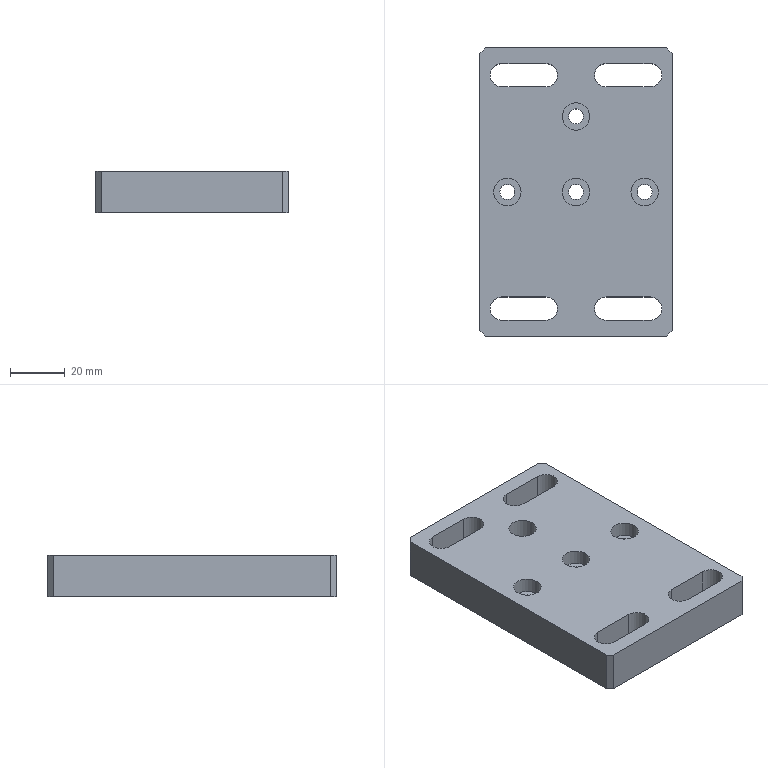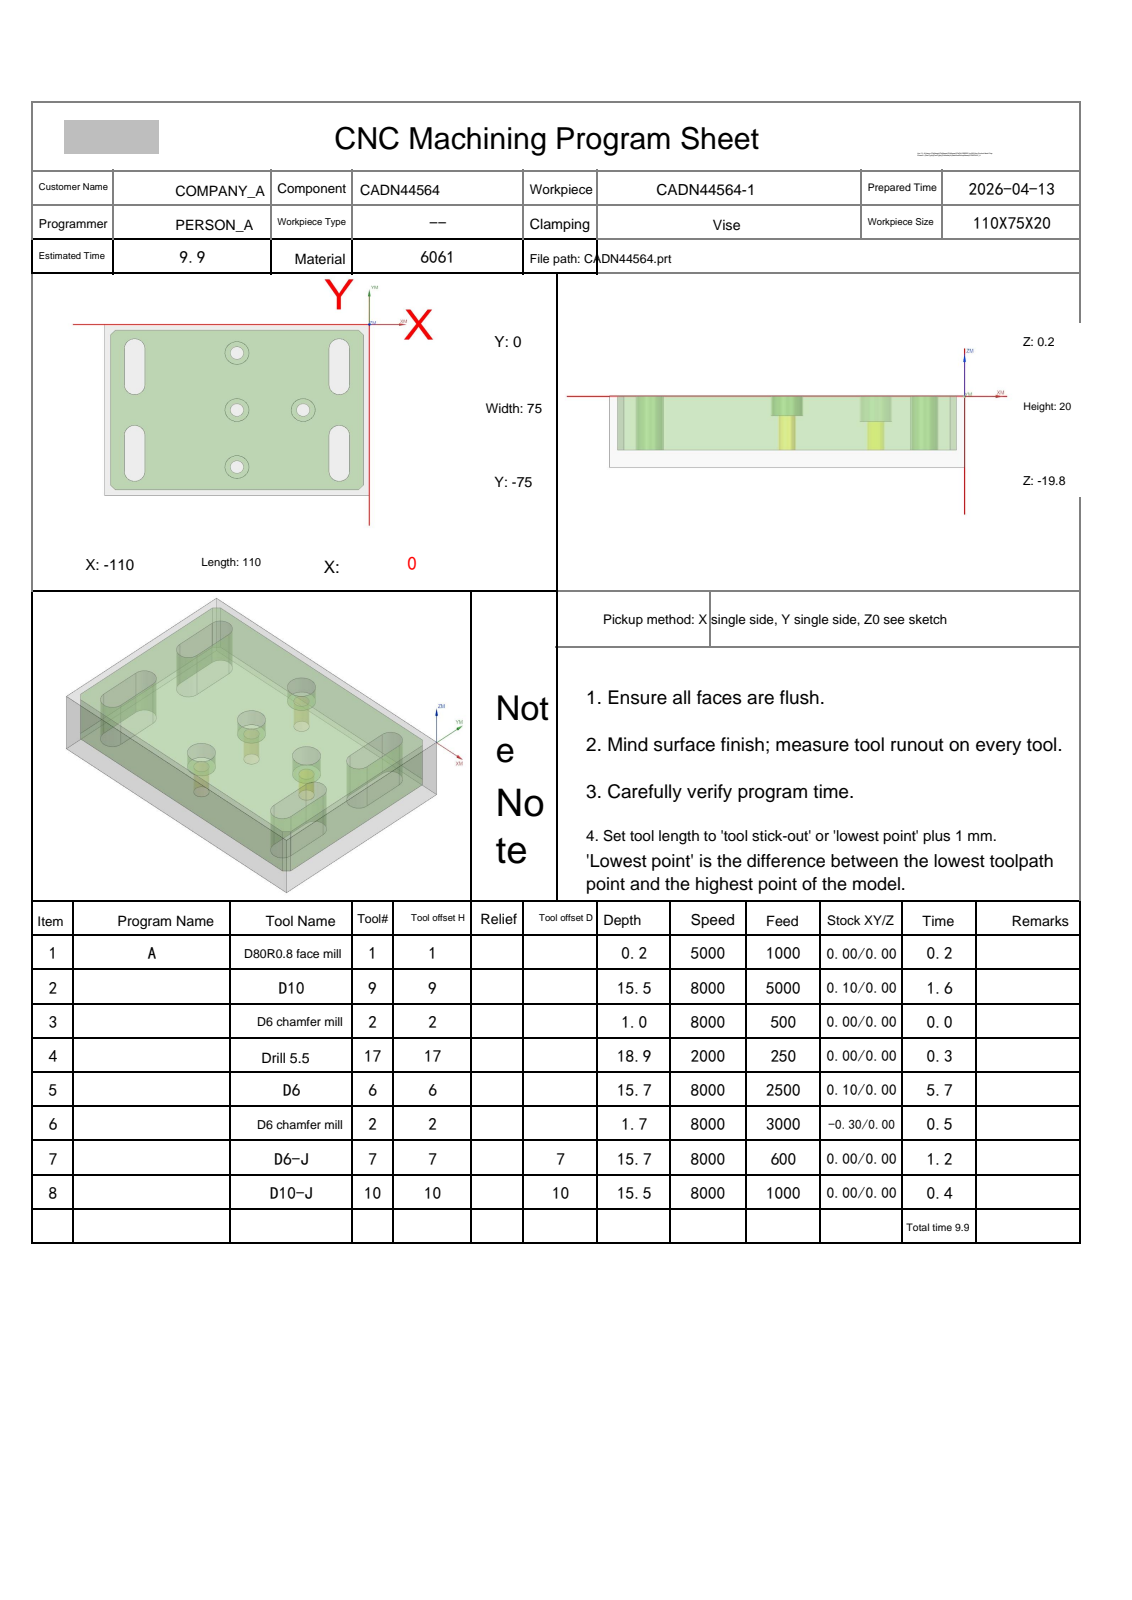NC program | NX | posted by the shop | part box 70 x 105 x 15 mm
Lines 1 to 417 of 3183:
%
O0001
(Machine time: 11.47 MIN)
(===Total Tool:7===)
(T1=D80R0.8 face mill D=80.  R=0.8  D-  H01 Z=0.    )
(T9=D10     D=10.  R=0.   D-  H09 Z=-15.3 )
(T2=D6 chamfer mill   D=6.   R=0.   D-  H02 Z=-1.5  )
(T17=Drill 5.5  D=5.5  DR_a=118 D-  H17 Z=-18.65)
(T6=D6      D=6.   R=0.   D-  H06 Z=-15.5 )
(T7=D6-J    D=6.   R=0.   D7  H07 Z=-15.5 )
(T10=D10-J  D=10.  R=0.   D10 H10 Z=-15.3 )
G80 G90 G17 G49 G40
G91 G28 Z0
M01
N1 T01 M06
(D80R0.8 face mill  D=80. R=0.8 H=01 ce=0.00 di=0.00)
G00 G90 G54 X-152.5 Y-37.5 M03 S5000
G43 H01 Z20.
M08
Z2.
G01 Z0.0 F1000.
X-147.5
X37.5
X42.5
Z2.
G00 Z20.
G91 G28 Z0.0
M05
M09
G91 G28 Z0.0
M01
N2 T09 M06
(D10  D=10. R=0. H=09 ce=0.10 di=0.00)
G00 G90 G54 X-55. Y-77.6 M03 S8000
G43 H09 Z20.
M08
Z.5
G01 X-105.5 Z.394 F5000.
G02 X-109.106 Y-76.106 Z.386 I0.0 J5.1
G01 X-111.106 Y-74.106 Z.38
G02 X-112.6 Y-70.5 Z.372 I3.606 J3.606
G01 Y-4.5 Z.233
G02 X-111.106 Y-.894 Z.225 I5.1 J0.0
G01 X-109.106 Y1.106 Z.219
G02 X-105.5 Y2.6 Z.211 I3.606 J-3.606
G01 X-4.5 Z-.001
G02 X-.894 Y1.106 Z-.009 I0.0 J-5.1
G01 X1.106 Y-.894 Z-.015
G02 X2.6 Y-4.5 Z-.023 I-3.606 J-3.606
G01 Y-70.5 Z-.162
G02 X1.106 Y-74.106 Z-.17 I-5.1 J0.0
G01 X-.894 Y-76.106 Z-.176
G02 X-4.5 Y-77.6 Z-.184 I-3.606 J3.606
G01 X-105.5 Z-.396
G02 X-109.106 Y-76.106 Z-.404 I0.0 J5.1
G01 X-111.106 Y-74.106 Z-.41
G02 X-112.6 Y-70.5 Z-.418 I3.606 J3.606
G01 Y-4.5 Z-.557
G02 X-111.106 Y-.894 Z-.565 I5.1 J0.0
G01 X-109.106 Y1.106 Z-.571
G02 X-105.5 Y2.6 Z-.579 I3.606 J-3.606
G01 X-4.5 Z-.791
G02 X-.894 Y1.106 Z-.799 I0.0 J-5.1
G01 X1.106 Y-.894 Z-.805
G02 X2.6 Y-4.5 Z-.813 I-3.606 J-3.606
G01 Y-70.5 Z-.952
G02 X1.106 Y-74.106 Z-.96 I-5.1 J0.0
G01 X-.894 Y-76.106 Z-.966
G02 X-4.5 Y-77.6 Z-.974 I-3.606 J3.606
G01 X-105.5 Z-1.186
G02 X-109.106 Y-76.106 Z-1.194 I0.0 J5.1
G01 X-111.106 Y-74.106 Z-1.2
G02 X-112.6 Y-70.5 Z-1.208 I3.606 J3.606
G01 Y-4.5 Z-1.347
G02 X-111.106 Y-.894 Z-1.355 I5.1 J0.0
G01 X-109.106 Y1.106 Z-1.361
G02 X-105.5 Y2.6 Z-1.369 I3.606 J-3.606
G01 X-4.5 Z-1.581
G02 X-.894 Y1.106 Z-1.589 I0.0 J-5.1
G01 X1.106 Y-.894 Z-1.595
G02 X2.6 Y-4.5 Z-1.603 I-3.606 J-3.606
G01 Y-70.5 Z-1.742
G02 X1.106 Y-74.106 Z-1.75 I-5.1 J0.0
G01 X-.894 Y-76.106 Z-1.756
G02 X-4.5 Y-77.6 Z-1.764 I-3.606 J3.606
G01 X-105.5 Z-1.976
G02 X-109.106 Y-76.106 Z-1.984 I0.0 J5.1
G01 X-111.106 Y-74.106 Z-1.99
G02 X-112.6 Y-70.5 Z-1.998 I3.606 J3.606
G01 Y-4.5 Z-2.137
G02 X-111.106 Y-.894 Z-2.145 I5.1 J0.0
G01 X-109.106 Y1.106 Z-2.151
G02 X-105.5 Y2.6 Z-2.159 I3.606 J-3.606
G01 X-4.5 Z-2.371
G02 X-.894 Y1.106 Z-2.379 I0.0 J-5.1
G01 X1.106 Y-.894 Z-2.385
G02 X2.6 Y-4.5 Z-2.393 I-3.606 J-3.606
G01 Y-70.5 Z-2.532
G02 X1.106 Y-74.106 Z-2.54 I-5.1 J0.0
G01 X-.894 Y-76.106 Z-2.546
G02 X-4.5 Y-77.6 Z-2.554 I-3.606 J3.606
G01 X-105.5 Z-2.766
G02 X-109.106 Y-76.106 Z-2.774 I0.0 J5.1
G01 X-111.106 Y-74.106 Z-2.78
G02 X-112.6 Y-70.5 Z-2.788 I3.606 J3.606
G01 Y-4.5 Z-2.927
G02 X-111.106 Y-.894 Z-2.935 I5.1 J0.0
G01 X-109.106 Y1.106 Z-2.941
G02 X-105.5 Y2.6 Z-2.949 I3.606 J-3.606
G01 X-4.5 Z-3.161
G02 X-.894 Y1.106 Z-3.169 I0.0 J-5.1
G01 X1.106 Y-.894 Z-3.175
G02 X2.6 Y-4.5 Z-3.183 I-3.606 J-3.606
G01 Y-70.5 Z-3.322
G02 X1.106 Y-74.106 Z-3.33 I-5.1 J0.0
G01 X-.894 Y-76.106 Z-3.336
G02 X-4.5 Y-77.6 Z-3.344 I-3.606 J3.606
G01 X-105.5 Z-3.556
G02 X-109.106 Y-76.106 Z-3.564 I0.0 J5.1
G01 X-111.106 Y-74.106 Z-3.57
G02 X-112.6 Y-70.5 Z-3.578 I3.606 J3.606
G01 Y-4.5 Z-3.717
G02 X-111.106 Y-.894 Z-3.725 I5.1 J0.0
G01 X-109.106 Y1.106 Z-3.731
G02 X-105.5 Y2.6 Z-3.739 I3.606 J-3.606
G01 X-4.5 Z-3.951
G02 X-.894 Y1.106 Z-3.959 I0.0 J-5.1
G01 X1.106 Y-.894 Z-3.965
G02 X2.6 Y-4.5 Z-3.973 I-3.606 J-3.606
G01 Y-70.5 Z-4.112
G02 X1.106 Y-74.106 Z-4.12 I-5.1 J0.0
G01 X-.894 Y-76.106 Z-4.126
G02 X-4.5 Y-77.6 Z-4.134 I-3.606 J3.606
G01 X-105.5 Z-4.346
G02 X-109.106 Y-76.106 Z-4.354 I0.0 J5.1
G01 X-111.106 Y-74.106 Z-4.36
G02 X-112.6 Y-70.5 Z-4.368 I3.606 J3.606
G01 Y-4.5 Z-4.507
G02 X-111.106 Y-.894 Z-4.515 I5.1 J0.0
G01 X-109.106 Y1.106 Z-4.521
G02 X-105.5 Y2.6 Z-4.529 I3.606 J-3.606
G01 X-4.5 Z-4.741
G02 X-.894 Y1.106 Z-4.749 I0.0 J-5.1
G01 X1.106 Y-.894 Z-4.755
G02 X2.6 Y-4.5 Z-4.763 I-3.606 J-3.606
G01 Y-70.5 Z-4.902
G02 X1.106 Y-74.106 Z-4.91 I-5.1 J0.0
G01 X-.894 Y-76.106 Z-4.916
G02 X-4.5 Y-77.6 Z-4.924 I-3.606 J3.606
G01 X-105.5 Z-5.136
G02 X-109.106 Y-76.106 Z-5.144 I0.0 J5.1
G01 X-111.106 Y-74.106 Z-5.15
G02 X-112.6 Y-70.5 Z-5.158 I3.606 J3.606
G01 Y-4.5 Z-5.297
G02 X-111.106 Y-.894 Z-5.305 I5.1 J0.0
G01 X-109.106 Y1.106 Z-5.311
G02 X-105.5 Y2.6 Z-5.319 I3.606 J-3.606
G01 X-4.5 Z-5.531
G02 X-.894 Y1.106 Z-5.539 I0.0 J-5.1
G01 X1.106 Y-.894 Z-5.545
G02 X2.6 Y-4.5 Z-5.553 I-3.606 J-3.606
G01 Y-70.5 Z-5.692
G02 X1.106 Y-74.106 Z-5.7 I-5.1 J0.0
G01 X-.894 Y-76.106 Z-5.706
G02 X-4.5 Y-77.6 Z-5.714 I-3.606 J3.606
G01 X-105.5 Z-5.926
G02 X-109.106 Y-76.106 Z-5.934 I0.0 J5.1
G01 X-111.106 Y-74.106 Z-5.94
G02 X-112.6 Y-70.5 Z-5.948 I3.606 J3.606
G01 Y-4.5 Z-6.087
G02 X-111.106 Y-.894 Z-6.095 I5.1 J0.0
G01 X-109.106 Y1.106 Z-6.101
G02 X-105.5 Y2.6 Z-6.109 I3.606 J-3.606
G01 X-4.5 Z-6.321
G02 X-.894 Y1.106 Z-6.329 I0.0 J-5.1
G01 X1.106 Y-.894 Z-6.335
G02 X2.6 Y-4.5 Z-6.343 I-3.606 J-3.606
G01 Y-70.5 Z-6.482
G02 X1.106 Y-74.106 Z-6.49 I-5.1 J0.0
G01 X-.894 Y-76.106 Z-6.496
G02 X-4.5 Y-77.6 Z-6.504 I-3.606 J3.606
G01 X-105.5 Z-6.716
G02 X-109.106 Y-76.106 Z-6.724 I0.0 J5.1
G01 X-111.106 Y-74.106 Z-6.73
G02 X-112.6 Y-70.5 Z-6.738 I3.606 J3.606
G01 Y-4.5 Z-6.877
G02 X-111.106 Y-.894 Z-6.885 I5.1 J0.0
G01 X-109.106 Y1.106 Z-6.891
G02 X-105.5 Y2.6 Z-6.899 I3.606 J-3.606
G01 X-4.5 Z-7.111
G02 X-.894 Y1.106 Z-7.119 I0.0 J-5.1
G01 X1.106 Y-.894 Z-7.125
G02 X2.6 Y-4.5 Z-7.133 I-3.606 J-3.606
G01 Y-70.5 Z-7.272
G02 X1.106 Y-74.106 Z-7.28 I-5.1 J0.0
G01 X-.894 Y-76.106 Z-7.286
G02 X-4.5 Y-77.6 Z-7.294 I-3.606 J3.606
G01 X-105.5 Z-7.506
G02 X-109.106 Y-76.106 Z-7.514 I0.0 J5.1
G01 X-111.106 Y-74.106 Z-7.52
G02 X-112.6 Y-70.5 Z-7.528 I3.606 J3.606
G01 Y-4.5 Z-7.667
G02 X-111.106 Y-.894 Z-7.675 I5.1 J0.0
G01 X-109.106 Y1.106 Z-7.681
G02 X-105.5 Y2.6 Z-7.689 I3.606 J-3.606
G01 X-4.5 Z-7.901
G02 X-.894 Y1.106 Z-7.909 I0.0 J-5.1
G01 X1.106 Y-.894 Z-7.915
G02 X2.6 Y-4.5 Z-7.923 I-3.606 J-3.606
G01 Y-70.5 Z-8.062
G02 X1.106 Y-74.106 Z-8.07 I-5.1 J0.0
G01 X-.894 Y-76.106 Z-8.076
G02 X-4.5 Y-77.6 Z-8.084 I-3.606 J3.606
G01 X-105.5 Z-8.296
G02 X-109.106 Y-76.106 Z-8.304 I0.0 J5.1
G01 X-111.106 Y-74.106 Z-8.31
G02 X-112.6 Y-70.5 Z-8.318 I3.606 J3.606
G01 Y-4.5 Z-8.457
G02 X-111.106 Y-.894 Z-8.465 I5.1 J0.0
G01 X-109.106 Y1.106 Z-8.471
G02 X-105.5 Y2.6 Z-8.479 I3.606 J-3.606
G01 X-4.5 Z-8.691
G02 X-.894 Y1.106 Z-8.699 I0.0 J-5.1
G01 X1.106 Y-.894 Z-8.705
G02 X2.6 Y-4.5 Z-8.713 I-3.606 J-3.606
G01 Y-70.5 Z-8.852
G02 X1.106 Y-74.106 Z-8.86 I-5.1 J0.0
G01 X-.894 Y-76.106 Z-8.866
G02 X-4.5 Y-77.6 Z-8.874 I-3.606 J3.606
G01 X-105.5 Z-9.086
G02 X-109.106 Y-76.106 Z-9.094 I0.0 J5.1
G01 X-111.106 Y-74.106 Z-9.1
G02 X-112.6 Y-70.5 Z-9.108 I3.606 J3.606
G01 Y-4.5 Z-9.247
G02 X-111.106 Y-.894 Z-9.255 I5.1 J0.0
G01 X-109.106 Y1.106 Z-9.261
G02 X-105.5 Y2.6 Z-9.269 I3.606 J-3.606
G01 X-4.5 Z-9.481
G02 X-.894 Y1.106 Z-9.489 I0.0 J-5.1
G01 X1.106 Y-.894 Z-9.495
G02 X2.6 Y-4.5 Z-9.503 I-3.606 J-3.606
G01 Y-70.5 Z-9.642
G02 X1.106 Y-74.106 Z-9.65 I-5.1 J0.0
G01 X-.894 Y-76.106 Z-9.656
G02 X-4.5 Y-77.6 Z-9.664 I-3.606 J3.606
G01 X-105.5 Z-9.876
G02 X-109.106 Y-76.106 Z-9.884 I0.0 J5.1
G01 X-111.106 Y-74.106 Z-9.89
G02 X-112.6 Y-70.5 Z-9.898 I3.606 J3.606
G01 Y-4.5 Z-10.037
G02 X-111.106 Y-.894 Z-10.045 I5.1 J0.0
G01 X-109.106 Y1.106 Z-10.051
G02 X-105.5 Y2.6 Z-10.059 I3.606 J-3.606
G01 X-4.5 Z-10.271
G02 X-.894 Y1.106 Z-10.279 I0.0 J-5.1
G01 X1.106 Y-.894 Z-10.285
G02 X2.6 Y-4.5 Z-10.293 I-3.606 J-3.606
G01 Y-70.5 Z-10.432
G02 X1.106 Y-74.106 Z-10.44 I-5.1 J0.0
G01 X-.894 Y-76.106 Z-10.446
G02 X-4.5 Y-77.6 Z-10.454 I-3.606 J3.606
G01 X-105.5 Z-10.666
G02 X-109.106 Y-76.106 Z-10.674 I0.0 J5.1
G01 X-111.106 Y-74.106 Z-10.68
G02 X-112.6 Y-70.5 Z-10.688 I3.606 J3.606
G01 Y-4.5 Z-10.827
G02 X-111.106 Y-.894 Z-10.835 I5.1 J0.0
G01 X-109.106 Y1.106 Z-10.841
G02 X-105.5 Y2.6 Z-10.849 I3.606 J-3.606
G01 X-4.5 Z-11.061
G02 X-.894 Y1.106 Z-11.069 I0.0 J-5.1
G01 X1.106 Y-.894 Z-11.075
G02 X2.6 Y-4.5 Z-11.083 I-3.606 J-3.606
G01 Y-70.5 Z-11.222
G02 X1.106 Y-74.106 Z-11.23 I-5.1 J0.0
G01 X-.894 Y-76.106 Z-11.236
G02 X-4.5 Y-77.6 Z-11.244 I-3.606 J3.606
G01 X-105.5 Z-11.456
G02 X-109.106 Y-76.106 Z-11.464 I0.0 J5.1
G01 X-111.106 Y-74.106 Z-11.47
G02 X-112.6 Y-70.5 Z-11.478 I3.606 J3.606
G01 Y-4.5 Z-11.617
G02 X-111.106 Y-.894 Z-11.625 I5.1 J0.0
G01 X-109.106 Y1.106 Z-11.631
G02 X-105.5 Y2.6 Z-11.639 I3.606 J-3.606
G01 X-4.5 Z-11.851
G02 X-.894 Y1.106 Z-11.859 I0.0 J-5.1
G01 X1.106 Y-.894 Z-11.865
G02 X2.6 Y-4.5 Z-11.873 I-3.606 J-3.606
G01 Y-70.5 Z-12.012
G02 X1.106 Y-74.106 Z-12.02 I-5.1 J0.0
G01 X-.894 Y-76.106 Z-12.026
G02 X-4.5 Y-77.6 Z-12.034 I-3.606 J3.606
G01 X-105.5 Z-12.246
G02 X-109.106 Y-76.106 Z-12.254 I0.0 J5.1
G01 X-111.106 Y-74.106 Z-12.26
G02 X-112.6 Y-70.5 Z-12.268 I3.606 J3.606
G01 Y-4.5 Z-12.407
G02 X-111.106 Y-.894 Z-12.415 I5.1 J0.0
G01 X-109.106 Y1.106 Z-12.421
G02 X-105.5 Y2.6 Z-12.429 I3.606 J-3.606
G01 X-4.5 Z-12.641
G02 X-.894 Y1.106 Z-12.649 I0.0 J-5.1
G01 X1.106 Y-.894 Z-12.655
G02 X2.6 Y-4.5 Z-12.663 I-3.606 J-3.606
G01 Y-70.5 Z-12.802
G02 X1.106 Y-74.106 Z-12.81 I-5.1 J0.0
G01 X-.894 Y-76.106 Z-12.816
G02 X-4.5 Y-77.6 Z-12.824 I-3.606 J3.606
G01 X-105.5 Z-13.036
G02 X-109.106 Y-76.106 Z-13.044 I0.0 J5.1
G01 X-111.106 Y-74.106 Z-13.05
G02 X-112.6 Y-70.5 Z-13.058 I3.606 J3.606
G01 Y-4.5 Z-13.197
G02 X-111.106 Y-.894 Z-13.205 I5.1 J0.0
G01 X-109.106 Y1.106 Z-13.211
G02 X-105.5 Y2.6 Z-13.219 I3.606 J-3.606
G01 X-4.5 Z-13.431
G02 X-.894 Y1.106 Z-13.439 I0.0 J-5.1
G01 X1.106 Y-.894 Z-13.445
G02 X2.6 Y-4.5 Z-13.453 I-3.606 J-3.606
G01 Y-70.5 Z-13.592
G02 X1.106 Y-74.106 Z-13.6 I-5.1 J0.0
G01 X-.894 Y-76.106 Z-13.606
G02 X-4.5 Y-77.6 Z-13.614 I-3.606 J3.606
G01 X-105.5 Z-13.826
G02 X-109.106 Y-76.106 Z-13.834 I0.0 J5.1
G01 X-111.106 Y-74.106 Z-13.84
G02 X-112.6 Y-70.5 Z-13.848 I3.606 J3.606
G01 Y-4.5 Z-13.987
G02 X-111.106 Y-.894 Z-13.995 I5.1 J0.0
G01 X-109.106 Y1.106 Z-14.001
G02 X-105.5 Y2.6 Z-14.009 I3.606 J-3.606
G01 X-4.5 Z-14.221
G02 X-.894 Y1.106 Z-14.229 I0.0 J-5.1
G01 X1.106 Y-.894 Z-14.235
G02 X2.6 Y-4.5 Z-14.243 I-3.606 J-3.606
G01 Y-70.5 Z-14.382
G02 X1.106 Y-74.106 Z-14.39 I-5.1 J0.0
G01 X-.894 Y-76.106 Z-14.396
G02 X-4.5 Y-77.6 Z-14.404 I-3.606 J3.606
G01 X-105.5 Z-14.616
G02 X-109.106 Y-76.106 Z-14.624 I0.0 J5.1
G01 X-111.106 Y-74.106 Z-14.63
G02 X-112.6 Y-70.5 Z-14.638 I3.606 J3.606
G01 Y-4.5 Z-14.777
G02 X-111.106 Y-.894 Z-14.785 I5.1 J0.0
G01 X-109.106 Y1.106 Z-14.791
G02 X-105.5 Y2.6 Z-14.799 I3.606 J-3.606
G01 X-4.5 Z-15.011
G02 X-.894 Y1.106 Z-15.019 I0.0 J-5.1
G01 X1.106 Y-.894 Z-15.025
G02 X2.6 Y-4.5 Z-15.033 I-3.606 J-3.606
G01 Y-70.5 Z-15.172
G02 X1.106 Y-74.106 Z-15.18 I-5.1 J0.0
G01 X-.894 Y-76.106 Z-15.186
G02 X-4.5 Y-77.6 Z-15.194 I-3.606 J3.606
G01 X-55. Z-15.3
X-105.5
G02 X-109.106 Y-76.106 I0.0 J5.1
G01 X-111.106 Y-74.106
G02 X-112.6 Y-70.5 I3.606 J3.606
G01 Y-4.5
G02 X-111.106 Y-.894 I5.1 J0.0
G01 X-109.106 Y1.106
G02 X-105.5 Y2.6 I3.606 J-3.606
G01 X-4.5
G02 X-.894 Y1.106 I0.0 J-5.1
G01 X1.106 Y-.894
G02 X2.6 Y-4.5 I-3.606 J-3.606
G01 Y-70.5
G02 X1.106 Y-74.106 I-5.1 J0.0
G01 X-.894 Y-76.106
G02 X-4.5 Y-77.6 I-3.606 J3.606
G01 X-55.
X-55.5
Z-14.3
G00 Z20.
G91 G28 Z0.0
M05
M09
G91 G28 Z0.0
M01
N3 T02 M06
(D6 chamfer mill  D=6. R=0. H=02 ce=0.00 di=0.00)
G00 G90 G54 X-27.5 Y-37.5 M03 S8000
G43 H02 Z20.
M08
G98 G81 X-27.5 Y-37.5 Z-.8 R1. F500.
X-55. Y-62.5
Y-37.5
Y-12.5
G80
G00 Z20.
G91 G28 Z0.0
M05
M09
G91 G28 Z0.0
M01
N4 T17 M06
(Drill 5.5 D=5.5 DR_a=118 H=17)
G00 G90 G54 X-27.5 Y-37.5 M03 S2000
G43 H17 Z20.
M08
G98 G83 X-27.5 Y-37.5 Z-18.652 R1. F250. Q2.
X-55. Y-62.5
Y-37.5
Y-12.5
G80
G00 Z20.
G91 G28 Z0.0
M05
M09
G91 G28 Z0.0
M01